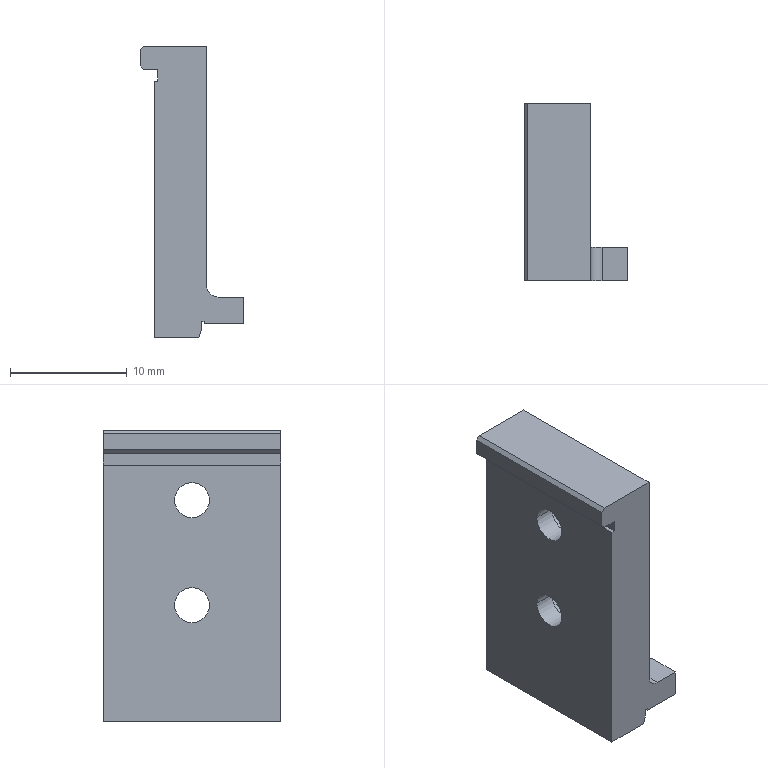Part | NX | 1 solid | 31 faces | box 8.9 x 15.2 x 25 mm | volume 1621 mm3 | plane 22 | cylinder 9 | commonest cylinder face diameters 3 x4 5 x4 2 x1
STEP:
#1=CARTESIAN_POINT('',(-1.77,0.,-1.43));
#2=VERTEX_POINT('',#1);
#3=CARTESIAN_POINT('',(-2.025,0.,-2.13));
#4=VERTEX_POINT('',#3);
#5=CARTESIAN_POINT('',(-1.25,0.,0.));
#6=DIRECTION('',(-0.342,0.,-0.9397));
#7=VECTOR('',#6,1000.);
#8=LINE('',#5,#7);
#9=EDGE_CURVE('',#2,#4,#8,.T.);
#10=ORIENTED_EDGE('',*,*,#9,.T.);
#11=CARTESIAN_POINT('',(-5.85,0.,-2.13));
#12=VERTEX_POINT('',#11);
#13=CARTESIAN_POINT('',(0.,0.,-2.13));
#14=DIRECTION('',(-1.,0.,0.));
#15=VECTOR('',#14,1000.);
#16=LINE('',#13,#15);
#17=EDGE_CURVE('',#4,#12,#16,.T.);
#18=ORIENTED_EDGE('',*,*,#17,.T.);
#19=CARTESIAN_POINT('',(-5.85,0.,19.87));
#20=VERTEX_POINT('',#19);
#21=CARTESIAN_POINT('',(-5.85,0.,0.));
#22=DIRECTION('',(0.,0.,-1.));
#23=VECTOR('',#22,1000.);
#24=LINE('',#21,#23);
#25=EDGE_CURVE('',#20,#12,#24,.T.);
#26=ORIENTED_EDGE('',*,*,#25,.F.);
#27=CARTESIAN_POINT('',(-5.55,0.,19.87));
#28=VERTEX_POINT('',#27);
#29=CARTESIAN_POINT('',(0.,0.,19.87));
#30=DIRECTION('',(-1.,0.,0.));
#31=VECTOR('',#30,1000.);
#32=LINE('',#29,#31);
#33=EDGE_CURVE('',#28,#20,#32,.T.);
#34=ORIENTED_EDGE('',*,*,#33,.F.);
#35=CARTESIAN_POINT('',(-5.55,0.,20.87));
#36=VERTEX_POINT('',#35);
#37=CARTESIAN_POINT('',(-5.55,0.,0.));
#38=DIRECTION('',(0.,0.,-1.));
#39=VECTOR('',#38,1000.);
#40=LINE('',#37,#39);
#41=EDGE_CURVE('',#36,#28,#40,.T.);
#42=ORIENTED_EDGE('',*,*,#41,.F.);
#43=CARTESIAN_POINT('',(-6.75,0.,20.87));
#44=VERTEX_POINT('',#43);
#45=CARTESIAN_POINT('',(0.,0.,20.87));
#46=DIRECTION('',(1.,0.,0.));
#47=VECTOR('',#46,1000.);
#48=LINE('',#45,#47);
#49=EDGE_CURVE('',#44,#36,#48,.T.);
#50=ORIENTED_EDGE('',*,*,#49,.F.);
#51=CARTESIAN_POINT('',(-7.05,0.,21.17));
#52=VERTEX_POINT('',#51);
#53=CARTESIAN_POINT('',(14.12,0.,0.));
#54=DIRECTION('',(0.7071,0.,-0.7071));
#55=VECTOR('',#54,1000.);
#56=LINE('',#53,#55);
#57=EDGE_CURVE('',#52,#44,#56,.T.);
#58=ORIENTED_EDGE('',*,*,#57,.F.);
#59=CARTESIAN_POINT('',(-7.05,0.,22.57));
#60=VERTEX_POINT('',#59);
#61=CARTESIAN_POINT('',(-7.05,0.,0.));
#62=DIRECTION('',(0.,0.,-1.));
#63=VECTOR('',#62,1000.);
#64=LINE('',#61,#63);
#65=EDGE_CURVE('',#60,#52,#64,.T.);
#66=ORIENTED_EDGE('',*,*,#65,.F.);
#67=CARTESIAN_POINT('',(-6.75,0.,22.87));
#68=VERTEX_POINT('',#67);
#69=CARTESIAN_POINT('',(-29.62,0.,0.));
#70=DIRECTION('',(0.7071,0.,0.7071));
#71=VECTOR('',#70,1000.);
#72=LINE('',#69,#71);
#73=EDGE_CURVE('',#60,#68,#72,.T.);
#74=ORIENTED_EDGE('',*,*,#73,.T.);
#75=CARTESIAN_POINT('',(-1.35,0.,22.87));
#76=VERTEX_POINT('',#75);
#77=CARTESIAN_POINT('',(0.,0.,22.87));
#78=DIRECTION('',(-1.,0.,0.));
#79=VECTOR('',#78,1000.);
#80=LINE('',#77,#79);
#81=EDGE_CURVE('',#76,#68,#80,.T.);
#82=ORIENTED_EDGE('',*,*,#81,.F.);
#83=CARTESIAN_POINT('',(-1.35,0.,-0.93));
#84=VERTEX_POINT('',#83);
#85=CARTESIAN_POINT('',(-1.35,0.,0.));
#86=DIRECTION('',(0.,0.,-1.));
#87=VECTOR('',#86,1000.);
#88=LINE('',#85,#87);
#89=EDGE_CURVE('',#76,#84,#88,.T.);
#90=ORIENTED_EDGE('',*,*,#89,.T.);
#91=CARTESIAN_POINT('',(-1.57,0.,-0.93));
#92=VERTEX_POINT('',#91);
#93=CARTESIAN_POINT('',(0.,0.,-0.93));
#94=DIRECTION('',(1.,0.,0.));
#95=VECTOR('',#94,1000.);
#96=LINE('',#93,#95);
#97=EDGE_CURVE('',#92,#84,#96,.T.);
#98=ORIENTED_EDGE('',*,*,#97,.F.);
#99=CARTESIAN_POINT('',(-1.57,0.,-0.73));
#100=VERTEX_POINT('',#99);
#101=CARTESIAN_POINT('',(-1.57,0.,0.));
#102=DIRECTION('',(0.,0.,1.));
#103=VECTOR('',#102,1000.);
#104=LINE('',#101,#103);
#105=EDGE_CURVE('',#92,#100,#104,.T.);
#106=ORIENTED_EDGE('',*,*,#105,.T.);
#107=CARTESIAN_POINT('',(-1.77,0.,-0.73));
#108=VERTEX_POINT('',#107);
#109=CARTESIAN_POINT('',(0.,0.,-0.73));
#110=DIRECTION('',(-1.,0.,0.));
#111=VECTOR('',#110,1000.);
#112=LINE('',#109,#111);
#113=EDGE_CURVE('',#100,#108,#112,.T.);
#114=ORIENTED_EDGE('',*,*,#113,.T.);
#115=CARTESIAN_POINT('',(-1.77,0.,0.));
#116=DIRECTION('',(0.,0.,-1.));
#117=VECTOR('',#116,1000.);
#118=LINE('',#115,#117);
#119=EDGE_CURVE('',#108,#2,#118,.T.);
#120=ORIENTED_EDGE('',*,*,#119,.T.);
#121=EDGE_LOOP('',(#10,#18,#26,#34,#42,#50,#58,#66,#74,#82,#90,#98,#106,#114,#120));
#122=FACE_BOUND('',#121,.T.);
#123=CARTESIAN_POINT('',(0.,0.,0.));
#124=DIRECTION('',(0.,-1.,0.));
#125=DIRECTION('',(0.,0.,-1.));
#126=AXIS2_PLACEMENT_3D('',#123,#124,#125);
#127=PLANE('',#126);
#128=ADVANCED_FACE('',(#122),#127,.F.);
#129=CARTESIAN_POINT('',(-1.77,-15.2,-1.43));
#130=VERTEX_POINT('',#129);
#131=CARTESIAN_POINT('',(-1.77,0.,-1.43));
#132=DIRECTION('',(0.,-1.,0.));
#133=VECTOR('',#132,1000.);
#134=LINE('',#131,#133);
#135=EDGE_CURVE('',#2,#130,#134,.T.);
#136=ORIENTED_EDGE('',*,*,#135,.F.);
#137=ORIENTED_EDGE('',*,*,#119,.F.);
#138=CARTESIAN_POINT('',(-1.77,-15.2,-0.73));
#139=VERTEX_POINT('',#138);
#140=CARTESIAN_POINT('',(-1.77,-15.2,-0.73));
#141=DIRECTION('',(0.,1.,0.));
#142=VECTOR('',#141,1000.);
#143=LINE('',#140,#142);
#144=EDGE_CURVE('',#139,#108,#143,.T.);
#145=ORIENTED_EDGE('',*,*,#144,.F.);
#146=CARTESIAN_POINT('',(-1.77,-15.2,0.));
#147=DIRECTION('',(0.,0.,1.));
#148=VECTOR('',#147,1000.);
#149=LINE('',#146,#148);
#150=EDGE_CURVE('',#130,#139,#149,.T.);
#151=ORIENTED_EDGE('',*,*,#150,.F.);
#152=EDGE_LOOP('',(#136,#137,#145,#151));
#153=FACE_BOUND('',#152,.T.);
#154=CARTESIAN_POINT('',(-1.77,0.,-0.93));
#155=DIRECTION('',(1.,0.,0.));
#156=DIRECTION('',(0.,1.,0.));
#157=AXIS2_PLACEMENT_3D('',#154,#155,#156);
#158=PLANE('',#157);
#159=ADVANCED_FACE('',(#153),#158,.T.);
#160=CARTESIAN_POINT('',(-0.35,-15.2,1.37));
#161=VERTEX_POINT('',#160);
#162=CARTESIAN_POINT('',(1.85,-15.2,1.37));
#163=VERTEX_POINT('',#162);
#164=CARTESIAN_POINT('',(0.,-15.2,1.37));
#165=DIRECTION('',(1.,0.,0.));
#166=VECTOR('',#165,1000.);
#167=LINE('',#164,#166);
#168=EDGE_CURVE('',#161,#163,#167,.T.);
#169=ORIENTED_EDGE('',*,*,#168,.F.);
#170=CARTESIAN_POINT('',(-1.35,-15.2,2.37));
#171=VERTEX_POINT('',#170);
#172=CARTESIAN_POINT('',(-0.35,-15.2,2.37));
#173=DIRECTION('',(0.,1.,0.));
#174=DIRECTION('',(-1.,0.,0.));
#175=AXIS2_PLACEMENT_3D('',#172,#173,#174);
#176=CIRCLE('',#175,1.);
#177=EDGE_CURVE('',#161,#171,#176,.T.);
#178=ORIENTED_EDGE('',*,*,#177,.T.);
#179=CARTESIAN_POINT('',(-1.35,-15.2,22.87));
#180=VERTEX_POINT('',#179);
#181=CARTESIAN_POINT('',(-1.35,-15.2,0.));
#182=DIRECTION('',(0.,0.,-1.));
#183=VECTOR('',#182,1000.);
#184=LINE('',#181,#183);
#185=EDGE_CURVE('',#180,#171,#184,.T.);
#186=ORIENTED_EDGE('',*,*,#185,.F.);
#187=CARTESIAN_POINT('',(-6.75,-15.2,22.87));
#188=VERTEX_POINT('',#187);
#189=CARTESIAN_POINT('',(0.,-15.2,22.87));
#190=DIRECTION('',(-1.,0.,0.));
#191=VECTOR('',#190,1000.);
#192=LINE('',#189,#191);
#193=EDGE_CURVE('',#180,#188,#192,.T.);
#194=ORIENTED_EDGE('',*,*,#193,.T.);
#195=CARTESIAN_POINT('',(-7.05,-15.2,22.57));
#196=VERTEX_POINT('',#195);
#197=CARTESIAN_POINT('',(-29.62,-15.2,0.));
#198=DIRECTION('',(-0.7071,0.,-0.7071));
#199=VECTOR('',#198,1000.);
#200=LINE('',#197,#199);
#201=EDGE_CURVE('',#188,#196,#200,.T.);
#202=ORIENTED_EDGE('',*,*,#201,.T.);
#203=CARTESIAN_POINT('',(-7.05,-15.2,21.17));
#204=VERTEX_POINT('',#203);
#205=CARTESIAN_POINT('',(-7.05,-15.2,0.));
#206=DIRECTION('',(0.,0.,-1.));
#207=VECTOR('',#206,1000.);
#208=LINE('',#205,#207);
#209=EDGE_CURVE('',#196,#204,#208,.T.);
#210=ORIENTED_EDGE('',*,*,#209,.T.);
#211=CARTESIAN_POINT('',(-6.75,-15.2,20.87));
#212=VERTEX_POINT('',#211);
#213=CARTESIAN_POINT('',(14.12,-15.2,0.));
#214=DIRECTION('',(-0.7071,0.,0.7071));
#215=VECTOR('',#214,1000.);
#216=LINE('',#213,#215);
#217=EDGE_CURVE('',#212,#204,#216,.T.);
#218=ORIENTED_EDGE('',*,*,#217,.F.);
#219=CARTESIAN_POINT('',(-5.55,-15.2,20.87));
#220=VERTEX_POINT('',#219);
#221=CARTESIAN_POINT('',(0.,-15.2,20.87));
#222=DIRECTION('',(1.,0.,0.));
#223=VECTOR('',#222,1000.);
#224=LINE('',#221,#223);
#225=EDGE_CURVE('',#212,#220,#224,.T.);
#226=ORIENTED_EDGE('',*,*,#225,.T.);
#227=CARTESIAN_POINT('',(-5.55,-15.2,19.87));
#228=VERTEX_POINT('',#227);
#229=CARTESIAN_POINT('',(-5.55,-15.2,0.));
#230=DIRECTION('',(0.,0.,-1.));
#231=VECTOR('',#230,1000.);
#232=LINE('',#229,#231);
#233=EDGE_CURVE('',#220,#228,#232,.T.);
#234=ORIENTED_EDGE('',*,*,#233,.T.);
#235=CARTESIAN_POINT('',(-5.85,-15.2,19.87));
#236=VERTEX_POINT('',#235);
#237=CARTESIAN_POINT('',(0.,-15.2,19.87));
#238=DIRECTION('',(-1.,0.,0.));
#239=VECTOR('',#238,1000.);
#240=LINE('',#237,#239);
#241=EDGE_CURVE('',#228,#236,#240,.T.);
#242=ORIENTED_EDGE('',*,*,#241,.T.);
#243=CARTESIAN_POINT('',(-5.85,-15.2,-2.13));
#244=VERTEX_POINT('',#243);
#245=CARTESIAN_POINT('',(-5.85,-15.2,0.));
#246=DIRECTION('',(0.,0.,-1.));
#247=VECTOR('',#246,1000.);
#248=LINE('',#245,#247);
#249=EDGE_CURVE('',#236,#244,#248,.T.);
#250=ORIENTED_EDGE('',*,*,#249,.T.);
#251=CARTESIAN_POINT('',(-2.025,-15.2,-2.13));
#252=VERTEX_POINT('',#251);
#253=CARTESIAN_POINT('',(0.,-15.2,-2.13));
#254=DIRECTION('',(-1.,0.,0.));
#255=VECTOR('',#254,1000.);
#256=LINE('',#253,#255);
#257=EDGE_CURVE('',#252,#244,#256,.T.);
#258=ORIENTED_EDGE('',*,*,#257,.F.);
#259=CARTESIAN_POINT('',(-1.25,-15.2,0.));
#260=DIRECTION('',(0.342,0.,0.9397));
#261=VECTOR('',#260,1000.);
#262=LINE('',#259,#261);
#263=EDGE_CURVE('',#252,#130,#262,.T.);
#264=ORIENTED_EDGE('',*,*,#263,.T.);
#265=ORIENTED_EDGE('',*,*,#150,.T.);
#266=CARTESIAN_POINT('',(-1.57,-15.2,-0.73));
#267=VERTEX_POINT('',#266);
#268=CARTESIAN_POINT('',(0.,-15.2,-0.73));
#269=DIRECTION('',(1.,0.,0.));
#270=VECTOR('',#269,1000.);
#271=LINE('',#268,#270);
#272=EDGE_CURVE('',#139,#267,#271,.T.);
#273=ORIENTED_EDGE('',*,*,#272,.T.);
#274=CARTESIAN_POINT('',(-1.57,-15.2,-0.93));
#275=VERTEX_POINT('',#274);
#276=CARTESIAN_POINT('',(-1.57,-15.2,0.));
#277=DIRECTION('',(0.,0.,-1.));
#278=VECTOR('',#277,1000.);
#279=LINE('',#276,#278);
#280=EDGE_CURVE('',#267,#275,#279,.T.);
#281=ORIENTED_EDGE('',*,*,#280,.T.);
#282=CARTESIAN_POINT('',(1.85,-15.2,-0.93));
#283=VERTEX_POINT('',#282);
#284=CARTESIAN_POINT('',(0.,-15.2,-0.93));
#285=DIRECTION('',(1.,0.,0.));
#286=VECTOR('',#285,1000.);
#287=LINE('',#284,#286);
#288=EDGE_CURVE('',#275,#283,#287,.T.);
#289=ORIENTED_EDGE('',*,*,#288,.T.);
#290=CARTESIAN_POINT('',(1.85,-15.2,0.));
#291=DIRECTION('',(0.,0.,-1.));
#292=VECTOR('',#291,1000.);
#293=LINE('',#290,#292);
#294=EDGE_CURVE('',#163,#283,#293,.T.);
#295=ORIENTED_EDGE('',*,*,#294,.F.);
#296=EDGE_LOOP('',(#169,#178,#186,#194,#202,#210,#218,#226,#234,#242,#250,#258,#264,#265,#273,#281,#289,#295));
#297=FACE_BOUND('',#296,.T.);
#298=CARTESIAN_POINT('',(-1.35,-15.2,0.));
#299=DIRECTION('',(0.,1.,0.));
#300=DIRECTION('',(1.,0.,0.));
#301=AXIS2_PLACEMENT_3D('',#298,#299,#300);
#302=PLANE('',#301);
#303=ADVANCED_FACE('',(#297),#302,.F.);
#304=CARTESIAN_POINT('',(-4.05,-5.1,7.87));
#305=VERTEX_POINT('',#304);
#306=CARTESIAN_POINT('',(-4.05,-10.1,7.87));
#307=VERTEX_POINT('',#306);
#308=CARTESIAN_POINT('',(-4.05,-7.6,7.87));
#309=DIRECTION('',(1.,0.,0.));
#310=DIRECTION('',(0.,-1.,0.));
#311=AXIS2_PLACEMENT_3D('',#308,#309,#310);
#312=CIRCLE('',#311,2.5);
#313=EDGE_CURVE('',#305,#307,#312,.T.);
#314=ORIENTED_EDGE('',*,*,#313,.T.);
#315=CARTESIAN_POINT('',(-4.05,-7.6,7.87));
#316=DIRECTION('',(1.,0.,0.));
#317=DIRECTION('',(0.,-1.,0.));
#318=AXIS2_PLACEMENT_3D('',#315,#316,#317);
#319=CIRCLE('',#318,2.5);
#320=EDGE_CURVE('',#307,#305,#319,.T.);
#321=ORIENTED_EDGE('',*,*,#320,.T.);
#322=EDGE_LOOP('',(#314,#321));
#323=FACE_BOUND('',#322,.T.);
#324=CARTESIAN_POINT('',(-4.05,-6.1,7.87));
#325=VERTEX_POINT('',#324);
#326=CARTESIAN_POINT('',(-4.05,-9.1,7.87));
#327=VERTEX_POINT('',#326);
#328=CARTESIAN_POINT('',(-4.05,-7.6,7.87));
#329=DIRECTION('',(1.,0.,0.));
#330=DIRECTION('',(0.,-1.,0.));
#331=AXIS2_PLACEMENT_3D('',#328,#329,#330);
#332=CIRCLE('',#331,1.5);
#333=EDGE_CURVE('',#325,#327,#332,.T.);
#334=ORIENTED_EDGE('',*,*,#333,.F.);
#335=CARTESIAN_POINT('',(-4.05,-7.6,7.87));
#336=DIRECTION('',(1.,0.,0.));
#337=DIRECTION('',(0.,-1.,0.));
#338=AXIS2_PLACEMENT_3D('',#335,#336,#337);
#339=CIRCLE('',#338,1.5);
#340=EDGE_CURVE('',#327,#325,#339,.T.);
#341=ORIENTED_EDGE('',*,*,#340,.F.);
#342=EDGE_LOOP('',(#334,#341));
#343=FACE_BOUND('',#342,.T.);
#344=CARTESIAN_POINT('',(-4.05,-7.6,7.87));
#345=DIRECTION('',(-1.,0.,0.));
#346=DIRECTION('',(0.,0.,1.));
#347=AXIS2_PLACEMENT_3D('',#344,#345,#346);
#348=PLANE('',#347);
#349=ADVANCED_FACE('',(#323,#343),#348,.F.);
#350=ORIENTED_EDGE('',*,*,#257,.T.);
#351=CARTESIAN_POINT('',(-5.85,0.,-2.13));
#352=DIRECTION('',(0.,1.,0.));
#353=VECTOR('',#352,1000.);
#354=LINE('',#351,#353);
#355=EDGE_CURVE('',#244,#12,#354,.T.);
#356=ORIENTED_EDGE('',*,*,#355,.T.);
#357=ORIENTED_EDGE('',*,*,#17,.F.);
#358=CARTESIAN_POINT('',(-2.025,0.,-2.13));
#359=DIRECTION('',(0.,-1.,0.));
#360=VECTOR('',#359,1000.);
#361=LINE('',#358,#360);
#362=EDGE_CURVE('',#4,#252,#361,.T.);
#363=ORIENTED_EDGE('',*,*,#362,.T.);
#364=EDGE_LOOP('',(#350,#356,#357,#363));
#365=FACE_BOUND('',#364,.T.);
#366=CARTESIAN_POINT('',(0.,0.,-2.13));
#367=DIRECTION('',(0.,0.,1.));
#368=DIRECTION('',(1.,0.,0.));
#369=AXIS2_PLACEMENT_3D('',#366,#367,#368);
#370=PLANE('',#369);
#371=ADVANCED_FACE('',(#365),#370,.F.);
#372=ORIENTED_EDGE('',*,*,#9,.F.);
#373=ORIENTED_EDGE('',*,*,#135,.T.);
#374=ORIENTED_EDGE('',*,*,#263,.F.);
#375=ORIENTED_EDGE('',*,*,#362,.F.);
#376=EDGE_LOOP('',(#372,#373,#374,#375));
#377=FACE_BOUND('',#376,.T.);
#378=CARTESIAN_POINT('',(-2.025,-15.2,-2.13));
#379=DIRECTION('',(0.9397,0.,-0.342));
#380=DIRECTION('',(0.,-1.,0.));
#381=AXIS2_PLACEMENT_3D('',#378,#379,#380);
#382=PLANE('',#381);
#383=ADVANCED_FACE('',(#377),#382,.T.);
#384=CARTESIAN_POINT('',(-5.85,0.,19.87));
#385=DIRECTION('',(0.,-1.,0.));
#386=VECTOR('',#385,1000.);
#387=LINE('',#384,#386);
#388=EDGE_CURVE('',#20,#236,#387,.T.);
#389=ORIENTED_EDGE('',*,*,#388,.T.);
#390=ORIENTED_EDGE('',*,*,#241,.F.);
#391=CARTESIAN_POINT('',(-5.55,0.,19.87));
#392=DIRECTION('',(0.,-1.,0.));
#393=VECTOR('',#392,1000.);
#394=LINE('',#391,#393);
#395=EDGE_CURVE('',#28,#228,#394,.T.);
#396=ORIENTED_EDGE('',*,*,#395,.F.);
#397=ORIENTED_EDGE('',*,*,#33,.T.);
#398=EDGE_LOOP('',(#389,#390,#396,#397));
#399=FACE_BOUND('',#398,.T.);
#400=CARTESIAN_POINT('',(-4.85,0.,19.87));
#401=DIRECTION('',(0.,0.,1.));
#402=DIRECTION('',(1.,0.,0.));
#403=AXIS2_PLACEMENT_3D('',#400,#401,#402);
#404=PLANE('',#403);
#405=ADVANCED_FACE('',(#399),#404,.T.);
#406=ORIENTED_EDGE('',*,*,#395,.T.);
#407=ORIENTED_EDGE('',*,*,#233,.F.);
#408=CARTESIAN_POINT('',(-5.55,0.,20.87));
#409=DIRECTION('',(0.,-1.,0.));
#410=VECTOR('',#409,1000.);
#411=LINE('',#408,#410);
#412=EDGE_CURVE('',#36,#220,#411,.T.);
#413=ORIENTED_EDGE('',*,*,#412,.F.);
#414=ORIENTED_EDGE('',*,*,#41,.T.);
#415=EDGE_LOOP('',(#406,#407,#413,#414));
#416=FACE_BOUND('',#415,.T.);
#417=CARTESIAN_POINT('',(-5.55,0.,19.87));
#418=DIRECTION('',(-1.,0.,0.));
#419=DIRECTION('',(0.,0.,1.));
#420=AXIS2_PLACEMENT_3D('',#417,#418,#419);
#421=PLANE('',#420);
#422=ADVANCED_FACE('',(#416),#421,.T.);
#423=CARTESIAN_POINT('',(-6.75,0.,20.87));
#424=DIRECTION('',(0.,1.,0.));
#425=VECTOR('',#424,1000.);
#426=LINE('',#423,#425);
#427=EDGE_CURVE('',#212,#44,#426,.T.);
#428=ORIENTED_EDGE('',*,*,#427,.T.);
#429=ORIENTED_EDGE('',*,*,#49,.T.);
#430=ORIENTED_EDGE('',*,*,#412,.T.);
#431=ORIENTED_EDGE('',*,*,#225,.F.);
#432=EDGE_LOOP('',(#428,#429,#430,#431));
#433=FACE_BOUND('',#432,.T.);
#434=CARTESIAN_POINT('',(-4.85,0.,20.87));
#435=DIRECTION('',(0.,0.,-1.));
#436=DIRECTION('',(0.,-1.,0.));
#437=AXIS2_PLACEMENT_3D('',#434,#435,#436);
#438=PLANE('',#437);
#439=ADVANCED_FACE('',(#433),#438,.T.);
#440=CARTESIAN_POINT('',(-7.05,0.,22.57));
#441=DIRECTION('',(0.,-1.,0.));
#442=VECTOR('',#441,1000.);
#443=LINE('',#440,#442);
#444=EDGE_CURVE('',#60,#196,#443,.T.);
#445=ORIENTED_EDGE('',*,*,#444,.F.);
#446=ORIENTED_EDGE('',*,*,#65,.T.);
#447=CARTESIAN_POINT('',(-7.05,0.,21.17));
#448=DIRECTION('',(0.,-1.,0.));
#449=VECTOR('',#448,1000.);
#450=LINE('',#447,#449);
#451=EDGE_CURVE('',#52,#204,#450,.T.);
#452=ORIENTED_EDGE('',*,*,#451,.T.);
#453=ORIENTED_EDGE('',*,*,#209,.F.);
#454=EDGE_LOOP('',(#445,#446,#452,#453));
#455=FACE_BOUND('',#454,.T.);
#456=CARTESIAN_POINT('',(-7.05,0.,20.87));
#457=DIRECTION('',(-1.,0.,0.));
#458=DIRECTION('',(0.,0.,1.));
#459=AXIS2_PLACEMENT_3D('',#456,#457,#458);
#460=PLANE('',#459);
#461=ADVANCED_FACE('',(#455),#460,.T.);
#462=CARTESIAN_POINT('',(-6.75,0.,22.87));
#463=DIRECTION('',(0.,1.,0.));
#464=VECTOR('',#463,1000.);
#465=LINE('',#462,#464);
#466=EDGE_CURVE('',#188,#68,#465,.T.);
#467=ORIENTED_EDGE('',*,*,#466,.F.);
#468=ORIENTED_EDGE('',*,*,#193,.F.);
#469=CARTESIAN_POINT('',(-1.35,0.,22.87));
#470=DIRECTION('',(0.,-1.,0.));
#471=VECTOR('',#470,1000.);
#472=LINE('',#469,#471);
#473=EDGE_CURVE('',#76,#180,#472,.T.);
#474=ORIENTED_EDGE('',*,*,#473,.F.);
#475=ORIENTED_EDGE('',*,*,#81,.T.);
#476=EDGE_LOOP('',(#467,#468,#474,#475));
#477=FACE_BOUND('',#476,.T.);
#478=CARTESIAN_POINT('',(-6.05,0.,22.87));
#479=DIRECTION('',(0.,0.,1.));
#480=DIRECTION('',(1.,0.,0.));
#481=AXIS2_PLACEMENT_3D('',#478,#479,#480);
#482=PLANE('',#481);
#483=ADVANCED_FACE('',(#477),#482,.T.);
#484=ORIENTED_EDGE('',*,*,#185,.T.);
#485=CARTESIAN_POINT('',(-1.35,-12.3,2.37));
#486=VERTEX_POINT('',#485);
#487=CARTESIAN_POINT('',(-1.35,-15.285,2.37));
#488=DIRECTION('',(0.,1.,0.));
#489=VECTOR('',#488,1000.);
#490=LINE('',#487,#489);
#491=EDGE_CURVE('',#171,#486,#490,.T.);
#492=ORIENTED_EDGE('',*,*,#491,.T.);
#493=CARTESIAN_POINT('',(-1.35,-12.3,-0.93));
#494=VERTEX_POINT('',#493);
#495=CARTESIAN_POINT('',(-1.35,-12.3,0.));
#496=DIRECTION('',(0.,0.,1.));
#497=VECTOR('',#496,1000.);
#498=LINE('',#495,#497);
#499=EDGE_CURVE('',#494,#486,#498,.T.);
#500=ORIENTED_EDGE('',*,*,#499,.F.);
#501=CARTESIAN_POINT('',(-1.35,0.,-0.93));
#502=DIRECTION('',(0.,-1.,0.));
#503=VECTOR('',#502,1000.);
#504=LINE('',#501,#503);
#505=EDGE_CURVE('',#84,#494,#504,.T.);
#506=ORIENTED_EDGE('',*,*,#505,.F.);
#507=ORIENTED_EDGE('',*,*,#89,.F.);
#508=ORIENTED_EDGE('',*,*,#473,.T.);
#509=EDGE_LOOP('',(#484,#492,#500,#506,#507,#508));
#510=FACE_BOUND('',#509,.T.);
#511=CARTESIAN_POINT('',(-1.35,-5.1,16.87));
#512=VERTEX_POINT('',#511);
#513=CARTESIAN_POINT('',(-1.35,-10.1,16.87));
#514=VERTEX_POINT('',#513);
#515=CARTESIAN_POINT('',(-1.35,-7.6,16.87));
#516=DIRECTION('',(1.,0.,0.));
#517=DIRECTION('',(0.,-1.,0.));
#518=AXIS2_PLACEMENT_3D('',#515,#516,#517);
#519=CIRCLE('',#518,2.5);
#520=EDGE_CURVE('',#512,#514,#519,.T.);
#521=ORIENTED_EDGE('',*,*,#520,.F.);
#522=CARTESIAN_POINT('',(-1.35,-7.6,16.87));
#523=DIRECTION('',(1.,0.,0.));
#524=DIRECTION('',(0.,-1.,0.));
#525=AXIS2_PLACEMENT_3D('',#522,#523,#524);
#526=CIRCLE('',#525,2.5);
#527=EDGE_CURVE('',#514,#512,#526,.T.);
#528=ORIENTED_EDGE('',*,*,#527,.F.);
#529=EDGE_LOOP('',(#521,#528));
#530=FACE_BOUND('',#529,.T.);
#531=CARTESIAN_POINT('',(-1.35,-10.1,7.87));
#532=VERTEX_POINT('',#531);
#533=CARTESIAN_POINT('',(-1.35,-5.1,7.87));
#534=VERTEX_POINT('',#533);
#535=CARTESIAN_POINT('',(-1.35,-7.6,7.87));
#536=DIRECTION('',(1.,0.,0.));
#537=DIRECTION('',(0.,-1.,0.));
#538=AXIS2_PLACEMENT_3D('',#535,#536,#537);
#539=CIRCLE('',#538,2.5);
#540=EDGE_CURVE('',#532,#534,#539,.T.);
#541=ORIENTED_EDGE('',*,*,#540,.F.);
#542=CARTESIAN_POINT('',(-1.35,-7.6,7.87));
#543=DIRECTION('',(1.,0.,0.));
#544=DIRECTION('',(0.,-1.,0.));
#545=AXIS2_PLACEMENT_3D('',#542,#543,#544);
#546=CIRCLE('',#545,2.5);
#547=EDGE_CURVE('',#534,#532,#546,.T.);
#548=ORIENTED_EDGE('',*,*,#547,.F.);
#549=EDGE_LOOP('',(#541,#548));
#550=FACE_BOUND('',#549,.T.);
#551=CARTESIAN_POINT('',(-1.35,0.,-1.13));
#552=DIRECTION('',(-1.,0.,0.));
#553=DIRECTION('',(0.,0.,1.));
#554=AXIS2_PLACEMENT_3D('',#551,#552,#553);
#555=PLANE('',#554);
#556=ADVANCED_FACE('',(#510,#530,#550),#555,.F.);
#557=ORIENTED_EDGE('',*,*,#491,.F.);
#558=ORIENTED_EDGE('',*,*,#177,.F.);
#559=CARTESIAN_POINT('',(-0.35,-12.3,1.37));
#560=VERTEX_POINT('',#559);
#561=CARTESIAN_POINT('',(-0.35,-15.2,1.37));
#562=DIRECTION('',(0.,1.,0.));
#563=VECTOR('',#562,1000.);
#564=LINE('',#561,#563);
#565=EDGE_CURVE('',#161,#560,#564,.T.);
#566=ORIENTED_EDGE('',*,*,#565,.T.);
#567=CARTESIAN_POINT('',(-0.35,-12.3,2.37));
#568=DIRECTION('',(0.,1.,0.));
#569=DIRECTION('',(-1.,0.,0.));
#570=AXIS2_PLACEMENT_3D('',#567,#568,#569);
#571=CIRCLE('',#570,1.);
#572=EDGE_CURVE('',#560,#486,#571,.T.);
#573=ORIENTED_EDGE('',*,*,#572,.T.);
#574=EDGE_LOOP('',(#557,#558,#566,#573));
#575=FACE_BOUND('',#574,.T.);
#576=CARTESIAN_POINT('',(-0.35,-15.285,2.37));
#577=DIRECTION('',(0.,1.,0.));
#578=DIRECTION('',(-1.,0.,0.));
#579=AXIS2_PLACEMENT_3D('',#576,#577,#578);
#580=CYLINDRICAL_SURFACE('',#579,1.);
#581=ADVANCED_FACE('',(#575),#580,.F.);
#582=CARTESIAN_POINT('',(1.85,-12.3,-0.93));
#583=VERTEX_POINT('',#582);
#584=CARTESIAN_POINT('',(1.85,-12.3,1.37));
#585=VERTEX_POINT('',#584);
#586=CARTESIAN_POINT('',(1.85,-12.3,0.));
#587=DIRECTION('',(0.,0.,1.));
#588=VECTOR('',#587,1000.);
#589=LINE('',#586,#588);
#590=EDGE_CURVE('',#583,#585,#589,.T.);
#591=ORIENTED_EDGE('',*,*,#590,.F.);
#592=CARTESIAN_POINT('',(0.,-12.3,-0.93));
#593=DIRECTION('',(-1.,0.,0.));
#594=VECTOR('',#593,1000.);
#595=LINE('',#592,#594);
#596=EDGE_CURVE('',#583,#494,#595,.T.);
#597=ORIENTED_EDGE('',*,*,#596,.T.);
#598=ORIENTED_EDGE('',*,*,#499,.T.);
#599=ORIENTED_EDGE('',*,*,#572,.F.);
#600=CARTESIAN_POINT('',(0.,-12.3,1.37));
#601=DIRECTION('',(-1.,0.,0.));
#602=VECTOR('',#601,1000.);
#603=LINE('',#600,#602);
#604=EDGE_CURVE('',#585,#560,#603,.T.);
#605=ORIENTED_EDGE('',*,*,#604,.F.);
#606=EDGE_LOOP('',(#591,#597,#598,#599,#605));
#607=FACE_BOUND('',#606,.T.);
#608=CARTESIAN_POINT('',(-1.77,-12.3,-0.83));
#609=DIRECTION('',(0.,-1.,0.));
#610=DIRECTION('',(0.,0.,-1.));
#611=AXIS2_PLACEMENT_3D('',#608,#609,#610);
#612=PLANE('',#611);
#613=ADVANCED_FACE('',(#607),#612,.F.);
#614=ORIENTED_EDGE('',*,*,#294,.T.);
#615=CARTESIAN_POINT('',(1.85,0.,-0.93));
#616=DIRECTION('',(0.,1.,0.));
#617=VECTOR('',#616,1000.);
#618=LINE('',#615,#617);
#619=EDGE_CURVE('',#283,#583,#618,.T.);
#620=ORIENTED_EDGE('',*,*,#619,.T.);
#621=ORIENTED_EDGE('',*,*,#590,.T.);
#622=CARTESIAN_POINT('',(1.85,0.,1.37));
#623=DIRECTION('',(0.,1.,0.));
#624=VECTOR('',#623,1000.);
#625=LINE('',#622,#624);
#626=EDGE_CURVE('',#163,#585,#625,.T.);
#627=ORIENTED_EDGE('',*,*,#626,.F.);
#628=EDGE_LOOP('',(#614,#620,#621,#627));
#629=FACE_BOUND('',#628,.T.);
#630=CARTESIAN_POINT('',(1.85,0.,52.77));
#631=DIRECTION('',(-1.,0.,0.));
#632=DIRECTION('',(0.,0.,1.));
#633=AXIS2_PLACEMENT_3D('',#630,#631,#632);
#634=PLANE('',#633);
#635=ADVANCED_FACE('',(#629),#634,.F.);
#636=ORIENTED_EDGE('',*,*,#540,.T.);
#637=CARTESIAN_POINT('',(-7.072,-5.1,7.87));
#638=DIRECTION('',(1.,0.,0.));
#639=VECTOR('',#638,1000.);
#640=LINE('',#637,#639);
#641=EDGE_CURVE('',#305,#534,#640,.T.);
#642=ORIENTED_EDGE('',*,*,#641,.F.);
#643=ORIENTED_EDGE('',*,*,#320,.F.);
#644=CARTESIAN_POINT('',(-7.072,-10.1,7.87));
#645=DIRECTION('',(1.,0.,0.));
#646=VECTOR('',#645,1000.);
#647=LINE('',#644,#646);
#648=EDGE_CURVE('',#307,#532,#647,.T.);
#649=ORIENTED_EDGE('',*,*,#648,.T.);
#650=EDGE_LOOP('',(#636,#642,#643,#649));
#651=FACE_BOUND('',#650,.T.);
#652=CARTESIAN_POINT('',(-7.072,-7.6,7.87));
#653=DIRECTION('',(1.,0.,0.));
#654=DIRECTION('',(0.,-1.,0.));
#655=AXIS2_PLACEMENT_3D('',#652,#653,#654);
#656=CYLINDRICAL_SURFACE('',#655,2.5);
#657=ADVANCED_FACE('',(#651),#656,.F.);
#658=ORIENTED_EDGE('',*,*,#604,.T.);
#659=ORIENTED_EDGE('',*,*,#565,.F.);
#660=ORIENTED_EDGE('',*,*,#168,.T.);
#661=ORIENTED_EDGE('',*,*,#626,.T.);
#662=EDGE_LOOP('',(#658,#659,#660,#661));
#663=FACE_BOUND('',#662,.T.);
#664=CARTESIAN_POINT('',(-1.35,-15.2,1.37));
#665=DIRECTION('',(0.,0.,-1.));
#666=DIRECTION('',(0.,-1.,0.));
#667=AXIS2_PLACEMENT_3D('',#664,#665,#666);
#668=PLANE('',#667);
#669=ADVANCED_FACE('',(#663),#668,.F.);
#670=ORIENTED_EDGE('',*,*,#97,.T.);
#671=ORIENTED_EDGE('',*,*,#505,.T.);
#672=ORIENTED_EDGE('',*,*,#596,.F.);
#673=ORIENTED_EDGE('',*,*,#619,.F.);
#674=ORIENTED_EDGE('',*,*,#288,.F.);
#675=CARTESIAN_POINT('',(-1.57,0.,-0.93));
#676=DIRECTION('',(0.,-1.,0.));
#677=VECTOR('',#676,1000.);
#678=LINE('',#675,#677);
#679=EDGE_CURVE('',#92,#275,#678,.T.);
#680=ORIENTED_EDGE('',*,*,#679,.F.);
#681=EDGE_LOOP('',(#670,#671,#672,#673,#674,#680));
#682=FACE_BOUND('',#681,.T.);
#683=CARTESIAN_POINT('',(1.45,0.,-0.93));
#684=DIRECTION('',(0.,0.,-1.));
#685=DIRECTION('',(0.,-1.,0.));
#686=AXIS2_PLACEMENT_3D('',#683,#684,#685);
#687=PLANE('',#686);
#688=ADVANCED_FACE('',(#682),#687,.T.);
#689=CARTESIAN_POINT('',(-1.57,-15.2,-0.73));
#690=DIRECTION('',(0.,1.,0.));
#691=VECTOR('',#690,1000.);
#692=LINE('',#689,#691);
#693=EDGE_CURVE('',#267,#100,#692,.T.);
#694=ORIENTED_EDGE('',*,*,#693,.T.);
#695=ORIENTED_EDGE('',*,*,#105,.F.);
#696=ORIENTED_EDGE('',*,*,#679,.T.);
#697=ORIENTED_EDGE('',*,*,#280,.F.);
#698=EDGE_LOOP('',(#694,#695,#696,#697));
#699=FACE_BOUND('',#698,.T.);
#700=CARTESIAN_POINT('',(-1.57,1.52,-0.93));
#701=DIRECTION('',(-1.,0.,0.));
#702=DIRECTION('',(0.,0.,1.));
#703=AXIS2_PLACEMENT_3D('',#700,#701,#702);
#704=PLANE('',#703);
#705=ADVANCED_FACE('',(#699),#704,.T.);
#706=ORIENTED_EDGE('',*,*,#144,.T.);
#707=ORIENTED_EDGE('',*,*,#113,.F.);
#708=ORIENTED_EDGE('',*,*,#693,.F.);
#709=ORIENTED_EDGE('',*,*,#272,.F.);
#710=EDGE_LOOP('',(#706,#707,#708,#709));
#711=FACE_BOUND('',#710,.T.);
#712=CARTESIAN_POINT('',(-1.57,1.52,-0.73));
#713=DIRECTION('',(0.,0.,-1.));
#714=DIRECTION('',(0.,-1.,0.));
#715=AXIS2_PLACEMENT_3D('',#712,#713,#714);
#716=PLANE('',#715);
#717=ADVANCED_FACE('',(#711),#716,.T.);
#718=CARTESIAN_POINT('',(-4.05,-10.1,16.87));
#719=VERTEX_POINT('',#718);
#720=CARTESIAN_POINT('',(-4.05,-5.1,16.87));
#721=VERTEX_POINT('',#720);
#722=CARTESIAN_POINT('',(-4.05,-7.6,16.87));
#723=DIRECTION('',(1.,0.,0.));
#724=DIRECTION('',(0.,-1.,0.));
#725=AXIS2_PLACEMENT_3D('',#722,#723,#724);
#726=CIRCLE('',#725,2.5);
#727=EDGE_CURVE('',#719,#721,#726,.T.);
#728=ORIENTED_EDGE('',*,*,#727,.F.);
#729=CARTESIAN_POINT('',(-7.072,-10.1,16.87));
#730=DIRECTION('',(1.,0.,0.));
#731=VECTOR('',#730,1000.);
#732=LINE('',#729,#731);
#733=EDGE_CURVE('',#514,#719,#732,.F.);
#734=ORIENTED_EDGE('',*,*,#733,.F.);
#735=ORIENTED_EDGE('',*,*,#527,.T.);
#736=CARTESIAN_POINT('',(-7.072,-5.1,16.87));
#737=DIRECTION('',(1.,0.,0.));
#738=VECTOR('',#737,1000.);
#739=LINE('',#736,#738);
#740=EDGE_CURVE('',#512,#721,#739,.F.);
#741=ORIENTED_EDGE('',*,*,#740,.T.);
#742=EDGE_LOOP('',(#728,#734,#735,#741));
#743=FACE_BOUND('',#742,.T.);
#744=CARTESIAN_POINT('',(-7.072,-7.6,16.87));
#745=DIRECTION('',(1.,0.,0.));
#746=DIRECTION('',(0.,-1.,0.));
#747=AXIS2_PLACEMENT_3D('',#744,#745,#746);
#748=CYLINDRICAL_SURFACE('',#747,2.5);
#749=ADVANCED_FACE('',(#743),#748,.F.);
#750=ORIENTED_EDGE('',*,*,#355,.F.);
#751=ORIENTED_EDGE('',*,*,#249,.F.);
#752=ORIENTED_EDGE('',*,*,#388,.F.);
#753=ORIENTED_EDGE('',*,*,#25,.T.);
#754=EDGE_LOOP('',(#750,#751,#752,#753));
#755=FACE_BOUND('',#754,.T.);
#756=CARTESIAN_POINT('',(-5.85,-6.1,16.87));
#757=VERTEX_POINT('',#756);
#758=CARTESIAN_POINT('',(-5.85,-9.1,16.87));
#759=VERTEX_POINT('',#758);
#760=CARTESIAN_POINT('',(-5.85,-7.6,16.87));
#761=DIRECTION('',(1.,0.,0.));
#762=DIRECTION('',(0.,-1.,0.));
#763=AXIS2_PLACEMENT_3D('',#760,#761,#762);
#764=CIRCLE('',#763,1.5);
#765=EDGE_CURVE('',#757,#759,#764,.T.);
#766=ORIENTED_EDGE('',*,*,#765,.T.);
#767=CARTESIAN_POINT('',(-5.85,-7.6,16.87));
#768=DIRECTION('',(1.,0.,0.));
#769=DIRECTION('',(0.,-1.,0.));
#770=AXIS2_PLACEMENT_3D('',#767,#768,#769);
#771=CIRCLE('',#770,1.5);
#772=EDGE_CURVE('',#759,#757,#771,.T.);
#773=ORIENTED_EDGE('',*,*,#772,.T.);
#774=EDGE_LOOP('',(#766,#773));
#775=FACE_BOUND('',#774,.T.);
#776=CARTESIAN_POINT('',(-5.85,-6.1,7.87));
#777=VERTEX_POINT('',#776);
#778=CARTESIAN_POINT('',(-5.85,-9.1,7.87));
#779=VERTEX_POINT('',#778);
#780=CARTESIAN_POINT('',(-5.85,-7.6,7.87));
#781=DIRECTION('',(1.,0.,0.));
#782=DIRECTION('',(0.,-1.,0.));
#783=AXIS2_PLACEMENT_3D('',#780,#781,#782);
#784=CIRCLE('',#783,1.5);
#785=EDGE_CURVE('',#777,#779,#784,.T.);
#786=ORIENTED_EDGE('',*,*,#785,.T.);
#787=CARTESIAN_POINT('',(-5.85,-7.6,7.87));
#788=DIRECTION('',(1.,0.,0.));
#789=DIRECTION('',(0.,-1.,0.));
#790=AXIS2_PLACEMENT_3D('',#787,#788,#789);
#791=CIRCLE('',#790,1.5);
#792=EDGE_CURVE('',#779,#777,#791,.T.);
#793=ORIENTED_EDGE('',*,*,#792,.T.);
#794=EDGE_LOOP('',(#786,#793));
#795=FACE_BOUND('',#794,.T.);
#796=CARTESIAN_POINT('',(-5.85,0.,-1.13));
#797=DIRECTION('',(-1.,0.,0.));
#798=DIRECTION('',(0.,0.,1.));
#799=AXIS2_PLACEMENT_3D('',#796,#797,#798);
#800=PLANE('',#799);
#801=ADVANCED_FACE('',(#755,#775,#795),#800,.T.);
#802=ORIENTED_EDGE('',*,*,#727,.T.);
#803=CARTESIAN_POINT('',(-4.05,-7.6,16.87));
#804=DIRECTION('',(1.,0.,0.));
#805=DIRECTION('',(0.,-1.,0.));
#806=AXIS2_PLACEMENT_3D('',#803,#804,#805);
#807=CIRCLE('',#806,2.5);
#808=EDGE_CURVE('',#721,#719,#807,.T.);
#809=ORIENTED_EDGE('',*,*,#808,.T.);
#810=EDGE_LOOP('',(#802,#809));
#811=FACE_BOUND('',#810,.T.);
#812=CARTESIAN_POINT('',(-4.05,-9.1,16.87));
#813=VERTEX_POINT('',#812);
#814=CARTESIAN_POINT('',(-4.05,-6.1,16.87));
#815=VERTEX_POINT('',#814);
#816=CARTESIAN_POINT('',(-4.05,-7.6,16.87));
#817=DIRECTION('',(1.,0.,0.));
#818=DIRECTION('',(0.,-1.,0.));
#819=AXIS2_PLACEMENT_3D('',#816,#817,#818);
#820=CIRCLE('',#819,1.5);
#821=EDGE_CURVE('',#813,#815,#820,.T.);
#822=ORIENTED_EDGE('',*,*,#821,.F.);
#823=CARTESIAN_POINT('',(-4.05,-7.6,16.87));
#824=DIRECTION('',(1.,0.,0.));
#825=DIRECTION('',(0.,-1.,0.));
#826=AXIS2_PLACEMENT_3D('',#823,#824,#825);
#827=CIRCLE('',#826,1.5);
#828=EDGE_CURVE('',#815,#813,#827,.T.);
#829=ORIENTED_EDGE('',*,*,#828,.F.);
#830=EDGE_LOOP('',(#822,#829));
#831=FACE_BOUND('',#830,.T.);
#832=CARTESIAN_POINT('',(-4.05,-7.6,16.87));
#833=DIRECTION('',(-1.,0.,0.));
#834=DIRECTION('',(0.,0.,1.));
#835=AXIS2_PLACEMENT_3D('',#832,#833,#834);
#836=PLANE('',#835);
#837=ADVANCED_FACE('',(#811,#831),#836,.F.);
#838=ORIENTED_EDGE('',*,*,#765,.F.);
#839=CARTESIAN_POINT('',(-7.072,-6.1,16.87));
#840=DIRECTION('',(1.,0.,0.));
#841=VECTOR('',#840,1000.);
#842=LINE('',#839,#841);
#843=EDGE_CURVE('',#757,#815,#842,.T.);
#844=ORIENTED_EDGE('',*,*,#843,.T.);
#845=ORIENTED_EDGE('',*,*,#828,.T.);
#846=CARTESIAN_POINT('',(-7.072,-9.1,16.87));
#847=DIRECTION('',(1.,0.,0.));
#848=VECTOR('',#847,1000.);
#849=LINE('',#846,#848);
#850=EDGE_CURVE('',#759,#813,#849,.T.);
#851=ORIENTED_EDGE('',*,*,#850,.F.);
#852=EDGE_LOOP('',(#838,#844,#845,#851));
#853=FACE_BOUND('',#852,.T.);
#854=CARTESIAN_POINT('',(-7.072,-7.6,16.87));
#855=DIRECTION('',(1.,0.,0.));
#856=DIRECTION('',(0.,-1.,0.));
#857=AXIS2_PLACEMENT_3D('',#854,#855,#856);
#858=CYLINDRICAL_SURFACE('',#857,1.5);
#859=ADVANCED_FACE('',(#853),#858,.F.);
#860=ORIENTED_EDGE('',*,*,#333,.T.);
#861=CARTESIAN_POINT('',(-7.072,-9.1,7.87));
#862=DIRECTION('',(1.,0.,0.));
#863=VECTOR('',#862,1000.);
#864=LINE('',#861,#863);
#865=EDGE_CURVE('',#327,#779,#864,.F.);
#866=ORIENTED_EDGE('',*,*,#865,.T.);
#867=ORIENTED_EDGE('',*,*,#785,.F.);
#868=CARTESIAN_POINT('',(-7.072,-6.1,7.87));
#869=DIRECTION('',(1.,0.,0.));
#870=VECTOR('',#869,1000.);
#871=LINE('',#868,#870);
#872=EDGE_CURVE('',#325,#777,#871,.F.);
#873=ORIENTED_EDGE('',*,*,#872,.F.);
#874=EDGE_LOOP('',(#860,#866,#867,#873));
#875=FACE_BOUND('',#874,.T.);
#876=CARTESIAN_POINT('',(-7.072,-7.6,7.87));
#877=DIRECTION('',(1.,0.,0.));
#878=DIRECTION('',(0.,-1.,0.));
#879=AXIS2_PLACEMENT_3D('',#876,#877,#878);
#880=CYLINDRICAL_SURFACE('',#879,1.5);
#881=ADVANCED_FACE('',(#875),#880,.F.);
#882=ORIENTED_EDGE('',*,*,#444,.T.);
#883=ORIENTED_EDGE('',*,*,#201,.F.);
#884=ORIENTED_EDGE('',*,*,#466,.T.);
#885=ORIENTED_EDGE('',*,*,#73,.F.);
#886=EDGE_LOOP('',(#882,#883,#884,#885));
#887=FACE_BOUND('',#886,.T.);
#888=CARTESIAN_POINT('',(-6.9,-7.6,22.72));
#889=DIRECTION('',(-0.7071,0.,0.7071));
#890=DIRECTION('',(0.,1.,0.));
#891=AXIS2_PLACEMENT_3D('',#888,#889,#890);
#892=PLANE('',#891);
#893=ADVANCED_FACE('',(#887),#892,.T.);
#894=ORIENTED_EDGE('',*,*,#427,.F.);
#895=ORIENTED_EDGE('',*,*,#217,.T.);
#896=ORIENTED_EDGE('',*,*,#451,.F.);
#897=ORIENTED_EDGE('',*,*,#57,.T.);
#898=EDGE_LOOP('',(#894,#895,#896,#897));
#899=FACE_BOUND('',#898,.T.);
#900=CARTESIAN_POINT('',(-6.9,-7.6,21.02));
#901=DIRECTION('',(0.7071,0.,0.7071));
#902=DIRECTION('',(0.,-1.,0.));
#903=AXIS2_PLACEMENT_3D('',#900,#901,#902);
#904=PLANE('',#903);
#905=ADVANCED_FACE('',(#899),#904,.F.);
#906=ORIENTED_EDGE('',*,*,#313,.F.);
#907=ORIENTED_EDGE('',*,*,#641,.T.);
#908=ORIENTED_EDGE('',*,*,#547,.T.);
#909=ORIENTED_EDGE('',*,*,#648,.F.);
#910=EDGE_LOOP('',(#906,#907,#908,#909));
#911=FACE_BOUND('',#910,.T.);
#912=CARTESIAN_POINT('',(-7.072,-7.6,7.87));
#913=DIRECTION('',(1.,0.,0.));
#914=DIRECTION('',(0.,-1.,0.));
#915=AXIS2_PLACEMENT_3D('',#912,#913,#914);
#916=CYLINDRICAL_SURFACE('',#915,2.5);
#917=ADVANCED_FACE('',(#911),#916,.F.);
#918=ORIENTED_EDGE('',*,*,#520,.T.);
#919=ORIENTED_EDGE('',*,*,#733,.T.);
#920=ORIENTED_EDGE('',*,*,#808,.F.);
#921=ORIENTED_EDGE('',*,*,#740,.F.);
#922=EDGE_LOOP('',(#918,#919,#920,#921));
#923=FACE_BOUND('',#922,.T.);
#924=CARTESIAN_POINT('',(-7.072,-7.6,16.87));
#925=DIRECTION('',(1.,0.,0.));
#926=DIRECTION('',(0.,-1.,0.));
#927=AXIS2_PLACEMENT_3D('',#924,#925,#926);
#928=CYLINDRICAL_SURFACE('',#927,2.5);
#929=ADVANCED_FACE('',(#923),#928,.F.);
#930=ORIENTED_EDGE('',*,*,#821,.T.);
#931=ORIENTED_EDGE('',*,*,#843,.F.);
#932=ORIENTED_EDGE('',*,*,#772,.F.);
#933=ORIENTED_EDGE('',*,*,#850,.T.);
#934=EDGE_LOOP('',(#930,#931,#932,#933));
#935=FACE_BOUND('',#934,.T.);
#936=CARTESIAN_POINT('',(-7.072,-7.6,16.87));
#937=DIRECTION('',(1.,0.,0.));
#938=DIRECTION('',(0.,-1.,0.));
#939=AXIS2_PLACEMENT_3D('',#936,#937,#938);
#940=CYLINDRICAL_SURFACE('',#939,1.5);
#941=ADVANCED_FACE('',(#935),#940,.F.);
#942=ORIENTED_EDGE('',*,*,#865,.F.);
#943=ORIENTED_EDGE('',*,*,#340,.T.);
#944=ORIENTED_EDGE('',*,*,#872,.T.);
#945=ORIENTED_EDGE('',*,*,#792,.F.);
#946=EDGE_LOOP('',(#942,#943,#944,#945));
#947=FACE_BOUND('',#946,.T.);
#948=CARTESIAN_POINT('',(-7.072,-7.6,7.87));
#949=DIRECTION('',(1.,0.,0.));
#950=DIRECTION('',(0.,-1.,0.));
#951=AXIS2_PLACEMENT_3D('',#948,#949,#950);
#952=CYLINDRICAL_SURFACE('',#951,1.5);
#953=ADVANCED_FACE('',(#947),#952,.F.);
#954=CLOSED_SHELL('',(#128,#159,#303,#349,#371,#383,#405,#422,#439,#461,#483,#556,#581,#613,#635,#657,#669,#688,#705,#717,#749,#801,#837,#859,#881,#893,#905,#917,#929,#941,#953));
#955=MANIFOLD_SOLID_BREP('',#954);
#956=(LENGTH_UNIT()NAMED_UNIT(*)SI_UNIT(.MILLI.,.METRE.));
#957=UNCERTAINTY_MEASURE_WITH_UNIT(LENGTH_MEASURE(0.00001),#956,'','');
#958=(NAMED_UNIT(*)PLANE_ANGLE_UNIT()SI_UNIT($,.RADIAN.));
#959=(NAMED_UNIT(*)SI_UNIT($,.STERADIAN.)SOLID_ANGLE_UNIT());
#960=(GEOMETRIC_REPRESENTATION_CONTEXT(3)GLOBAL_UNCERTAINTY_ASSIGNED_CONTEXT((#957))GLOBAL_UNIT_ASSIGNED_CONTEXT((#956,#958,#959))REPRESENTATION_CONTEXT('',''));
#961=ADVANCED_BREP_SHAPE_REPRESENTATION('',(#955),#960);